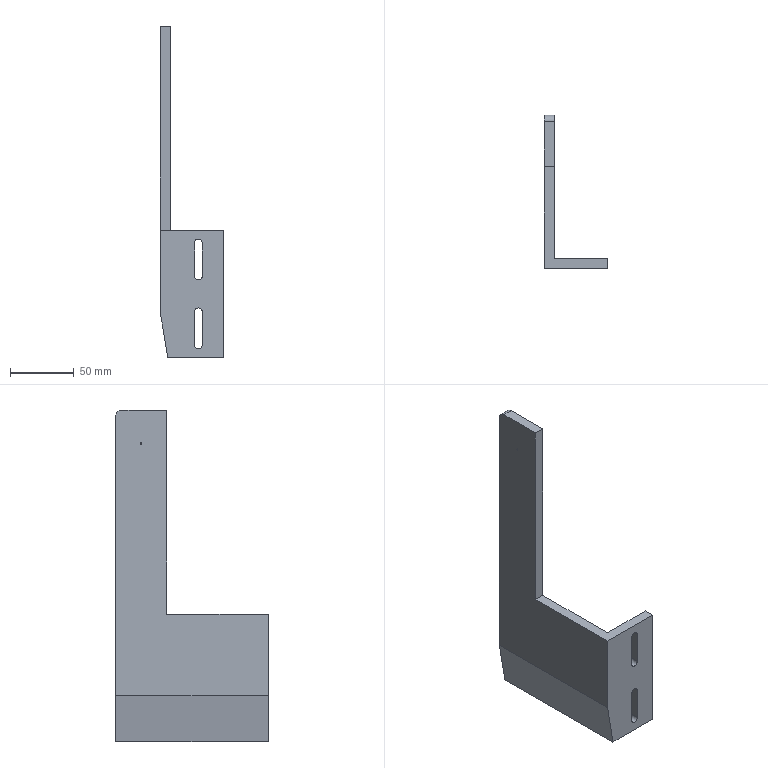Part | SolidWorks | features ICE 4, 3DProfileFeature 1, Extrusion 1, Fillet 1, HoleWzd 1 | 1 solid | 30 faces | box 50 x 120 x 260 mm | volume 164749 mm3 | plane 15 | cylinder 11 | cone 4 | commonest cylinder face diameters 6 x6 1.2 x2 4.2 x2 10 x1
STEP:
#1=CARTESIAN_POINT('',(0.,100.,234.6));
#2=VERTEX_POINT('',#1);
#3=CARTESIAN_POINT('',(0.,100.,233.4));
#4=VERTEX_POINT('',#3);
#5=CARTESIAN_POINT('',(0.,100.,234.));
#6=DIRECTION('',(1.,0.,0.));
#7=DIRECTION('',(0.,0.,-1.));
#8=AXIS2_PLACEMENT_3D('',#5,#6,#7);
#9=CIRCLE('',#8,0.6);
#10=EDGE_CURVE('',#2,#4,#9,.T.);
#11=ORIENTED_EDGE('',*,*,#10,.F.);
#12=CARTESIAN_POINT('',(8.,100.,234.6));
#13=VERTEX_POINT('',#12);
#14=CARTESIAN_POINT('',(0.,100.,234.6));
#15=DIRECTION('',(1.,0.,0.));
#16=VECTOR('',#15,1000.);
#17=LINE('',#14,#16);
#18=EDGE_CURVE('',#2,#13,#17,.T.);
#19=ORIENTED_EDGE('',*,*,#18,.T.);
#20=CARTESIAN_POINT('',(8.,100.,233.4));
#21=VERTEX_POINT('',#20);
#22=CARTESIAN_POINT('',(8.,100.,234.));
#23=DIRECTION('',(1.,0.,0.));
#24=DIRECTION('',(0.,0.,-1.));
#25=AXIS2_PLACEMENT_3D('',#22,#23,#24);
#26=CIRCLE('',#25,0.6);
#27=EDGE_CURVE('',#13,#21,#26,.T.);
#28=ORIENTED_EDGE('',*,*,#27,.T.);
#29=CARTESIAN_POINT('',(0.,100.,233.4));
#30=DIRECTION('',(1.,0.,0.));
#31=VECTOR('',#30,1000.);
#32=LINE('',#29,#31);
#33=EDGE_CURVE('',#4,#21,#32,.T.);
#34=ORIENTED_EDGE('',*,*,#33,.F.);
#35=EDGE_LOOP('',(#11,#19,#28,#34));
#36=FACE_OUTER_BOUND('',#35,.T.);
#37=CARTESIAN_POINT('',(0.,100.,234.));
#38=DIRECTION('',(1.,0.,0.));
#39=DIRECTION('',(0.,0.,-1.));
#40=AXIS2_PLACEMENT_3D('',#37,#38,#39);
#41=CYLINDRICAL_SURFACE('',#40,0.6);
#42=ADVANCED_FACE('',(#36),#41,.F.);
#43=CARTESIAN_POINT('',(7.575,75.,87.1));
#44=VERTEX_POINT('',#43);
#45=CARTESIAN_POINT('',(7.575,75.,82.9));
#46=VERTEX_POINT('',#45);
#47=CARTESIAN_POINT('',(7.575,75.,85.));
#48=DIRECTION('',(1.,0.,0.));
#49=DIRECTION('',(0.,0.,-1.));
#50=AXIS2_PLACEMENT_3D('',#47,#48,#49);
#51=CIRCLE('',#50,2.1);
#52=EDGE_CURVE('',#44,#46,#51,.T.);
#53=ORIENTED_EDGE('',*,*,#52,.F.);
#54=CARTESIAN_POINT('',(8.,75.,87.525));
#55=VERTEX_POINT('',#54);
#56=CARTESIAN_POINT('',(8.,75.,87.525));
#57=DIRECTION('',(0.7071,0.,0.7071));
#58=VECTOR('',#57,1000.);
#59=LINE('',#56,#58);
#60=EDGE_CURVE('',#44,#55,#59,.T.);
#61=ORIENTED_EDGE('',*,*,#60,.T.);
#62=CARTESIAN_POINT('',(8.,75.,82.475));
#63=VERTEX_POINT('',#62);
#64=CARTESIAN_POINT('',(8.,75.,85.));
#65=DIRECTION('',(1.,0.,0.));
#66=DIRECTION('',(0.,0.,-1.));
#67=AXIS2_PLACEMENT_3D('',#64,#65,#66);
#68=CIRCLE('',#67,2.525);
#69=EDGE_CURVE('',#55,#63,#68,.T.);
#70=ORIENTED_EDGE('',*,*,#69,.T.);
#71=CARTESIAN_POINT('',(8.,75.,82.475));
#72=DIRECTION('',(0.7071,0.,-0.7071));
#73=VECTOR('',#72,1000.);
#74=LINE('',#71,#73);
#75=EDGE_CURVE('',#46,#63,#74,.T.);
#76=ORIENTED_EDGE('',*,*,#75,.F.);
#77=EDGE_LOOP('',(#53,#61,#70,#76));
#78=FACE_OUTER_BOUND('',#77,.T.);
#79=CARTESIAN_POINT('',(8.,75.,85.));
#80=DIRECTION('',(1.,0.,0.));
#81=DIRECTION('',(0.,0.,-1.));
#82=AXIS2_PLACEMENT_3D('',#79,#80,#81);
#83=CONICAL_SURFACE('',#82,2.525,0.7854);
#84=ADVANCED_FACE('',(#78),#83,.F.);
#85=CARTESIAN_POINT('',(2.,75.,87.1));
#86=VERTEX_POINT('',#85);
#87=CARTESIAN_POINT('',(2.,75.,82.9));
#88=VERTEX_POINT('',#87);
#89=CARTESIAN_POINT('',(2.,75.,85.));
#90=DIRECTION('',(1.,0.,0.));
#91=DIRECTION('',(0.,0.,-1.));
#92=AXIS2_PLACEMENT_3D('',#89,#90,#91);
#93=CIRCLE('',#92,2.1);
#94=EDGE_CURVE('',#86,#88,#93,.T.);
#95=ORIENTED_EDGE('',*,*,#94,.F.);
#96=CARTESIAN_POINT('',(8.,75.,87.1));
#97=DIRECTION('',(1.,0.,0.));
#98=VECTOR('',#97,1000.);
#99=LINE('',#96,#98);
#100=EDGE_CURVE('',#86,#44,#99,.T.);
#101=ORIENTED_EDGE('',*,*,#100,.T.);
#102=ORIENTED_EDGE('',*,*,#52,.T.);
#103=CARTESIAN_POINT('',(8.,75.,82.9));
#104=DIRECTION('',(1.,0.,0.));
#105=VECTOR('',#104,1000.);
#106=LINE('',#103,#105);
#107=EDGE_CURVE('',#88,#46,#106,.T.);
#108=ORIENTED_EDGE('',*,*,#107,.F.);
#109=EDGE_LOOP('',(#95,#101,#102,#108));
#110=FACE_OUTER_BOUND('',#109,.T.);
#111=CARTESIAN_POINT('',(8.,75.,85.));
#112=DIRECTION('',(1.,0.,0.));
#113=DIRECTION('',(0.,0.,-1.));
#114=AXIS2_PLACEMENT_3D('',#111,#112,#113);
#115=CYLINDRICAL_SURFACE('',#114,2.1);
#116=ADVANCED_FACE('',(#110),#115,.F.);
#117=CARTESIAN_POINT('',(0.7382,75.,85.));
#118=VERTEX_POINT('',#117);
#119=CARTESIAN_POINT('',(2.,75.,82.9));
#120=DIRECTION('',(0.515,0.,-0.8572));
#121=VECTOR('',#120,1000.);
#122=LINE('',#119,#121);
#123=EDGE_CURVE('',#118,#88,#122,.T.);
#124=ORIENTED_EDGE('',*,*,#123,.F.);
#125=CARTESIAN_POINT('',(2.,75.,87.1));
#126=DIRECTION('',(0.515,0.,0.8572));
#127=VECTOR('',#126,1000.);
#128=LINE('',#125,#127);
#129=EDGE_CURVE('',#118,#86,#128,.T.);
#130=ORIENTED_EDGE('',*,*,#129,.T.);
#131=ORIENTED_EDGE('',*,*,#94,.T.);
#132=EDGE_LOOP('',(#124,#130,#131));
#133=FACE_OUTER_BOUND('',#132,.T.);
#134=CARTESIAN_POINT('',(2.,75.,85.));
#135=DIRECTION('',(1.,0.,0.));
#136=DIRECTION('',(0.,0.,-1.));
#137=AXIS2_PLACEMENT_3D('',#134,#135,#136);
#138=CONICAL_SURFACE('',#137,2.1,1.03);
#139=ADVANCED_FACE('',(#133),#138,.F.);
#140=CARTESIAN_POINT('',(30.,0.,39.));
#141=VERTEX_POINT('',#140);
#142=CARTESIAN_POINT('',(33.,0.,36.));
#143=VERTEX_POINT('',#142);
#144=CARTESIAN_POINT('',(30.,0.,36.));
#145=DIRECTION('',(0.,1.,0.));
#146=DIRECTION('',(0.,0.,1.));
#147=AXIS2_PLACEMENT_3D('',#144,#145,#146);
#148=CIRCLE('',#147,3.);
#149=EDGE_CURVE('',#141,#143,#148,.T.);
#150=ORIENTED_EDGE('',*,*,#149,.F.);
#151=CARTESIAN_POINT('',(30.,8.,39.));
#152=VERTEX_POINT('',#151);
#153=CARTESIAN_POINT('',(30.,-212.,39.));
#154=DIRECTION('',(0.,1.,0.));
#155=VECTOR('',#154,1000.);
#156=LINE('',#153,#155);
#157=EDGE_CURVE('',#141,#152,#156,.T.);
#158=ORIENTED_EDGE('',*,*,#157,.T.);
#159=CARTESIAN_POINT('',(33.,8.,36.));
#160=VERTEX_POINT('',#159);
#161=CARTESIAN_POINT('',(30.,8.,36.));
#162=DIRECTION('',(0.,1.,0.));
#163=DIRECTION('',(0.,0.,1.));
#164=AXIS2_PLACEMENT_3D('',#161,#162,#163);
#165=CIRCLE('',#164,3.);
#166=EDGE_CURVE('',#152,#160,#165,.T.);
#167=ORIENTED_EDGE('',*,*,#166,.T.);
#168=CARTESIAN_POINT('',(33.,-212.,36.));
#169=DIRECTION('',(0.,1.,0.));
#170=VECTOR('',#169,1000.);
#171=LINE('',#168,#170);
#172=EDGE_CURVE('',#143,#160,#171,.T.);
#173=ORIENTED_EDGE('',*,*,#172,.F.);
#174=EDGE_LOOP('',(#150,#158,#167,#173));
#175=FACE_OUTER_BOUND('',#174,.T.);
#176=CARTESIAN_POINT('',(30.,-212.,36.));
#177=DIRECTION('',(0.,1.,0.));
#178=DIRECTION('',(0.,0.,1.));
#179=AXIS2_PLACEMENT_3D('',#176,#177,#178);
#180=CYLINDRICAL_SURFACE('',#179,3.);
#181=ADVANCED_FACE('',(#175),#180,.F.);
#182=CARTESIAN_POINT('',(30.,0.,93.));
#183=VERTEX_POINT('',#182);
#184=CARTESIAN_POINT('',(33.,0.,90.));
#185=VERTEX_POINT('',#184);
#186=CARTESIAN_POINT('',(30.,0.,90.));
#187=DIRECTION('',(0.,1.,0.));
#188=DIRECTION('',(0.,0.,1.));
#189=AXIS2_PLACEMENT_3D('',#186,#187,#188);
#190=CIRCLE('',#189,3.);
#191=EDGE_CURVE('',#183,#185,#190,.T.);
#192=ORIENTED_EDGE('',*,*,#191,.F.);
#193=CARTESIAN_POINT('',(30.,8.,93.));
#194=VERTEX_POINT('',#193);
#195=CARTESIAN_POINT('',(30.,-212.,93.));
#196=DIRECTION('',(0.,1.,0.));
#197=VECTOR('',#196,1000.);
#198=LINE('',#195,#197);
#199=EDGE_CURVE('',#183,#194,#198,.T.);
#200=ORIENTED_EDGE('',*,*,#199,.T.);
#201=CARTESIAN_POINT('',(33.,8.,90.));
#202=VERTEX_POINT('',#201);
#203=CARTESIAN_POINT('',(30.,8.,90.));
#204=DIRECTION('',(0.,1.,0.));
#205=DIRECTION('',(0.,0.,1.));
#206=AXIS2_PLACEMENT_3D('',#203,#204,#205);
#207=CIRCLE('',#206,3.);
#208=EDGE_CURVE('',#194,#202,#207,.T.);
#209=ORIENTED_EDGE('',*,*,#208,.T.);
#210=CARTESIAN_POINT('',(33.,-212.,90.));
#211=DIRECTION('',(0.,1.,0.));
#212=VECTOR('',#211,1000.);
#213=LINE('',#210,#212);
#214=EDGE_CURVE('',#185,#202,#213,.T.);
#215=ORIENTED_EDGE('',*,*,#214,.F.);
#216=EDGE_LOOP('',(#192,#200,#209,#215));
#217=FACE_OUTER_BOUND('',#216,.T.);
#218=CARTESIAN_POINT('',(30.,-212.,90.));
#219=DIRECTION('',(0.,1.,0.));
#220=DIRECTION('',(0.,0.,1.));
#221=AXIS2_PLACEMENT_3D('',#218,#219,#220);
#222=CYLINDRICAL_SURFACE('',#221,3.);
#223=ADVANCED_FACE('',(#217),#222,.F.);
#224=CARTESIAN_POINT('',(27.,0.,10.));
#225=VERTEX_POINT('',#224);
#226=CARTESIAN_POINT('',(27.,0.,36.));
#227=VERTEX_POINT('',#226);
#228=CARTESIAN_POINT('',(27.,0.,260.));
#229=DIRECTION('',(0.,0.,1.));
#230=VECTOR('',#229,1000.);
#231=LINE('',#228,#230);
#232=EDGE_CURVE('',#225,#227,#231,.T.);
#233=ORIENTED_EDGE('',*,*,#232,.T.);
#234=CARTESIAN_POINT('',(30.,0.,36.));
#235=DIRECTION('',(0.,1.,0.));
#236=DIRECTION('',(0.,0.,1.));
#237=AXIS2_PLACEMENT_3D('',#234,#235,#236);
#238=CIRCLE('',#237,3.);
#239=EDGE_CURVE('',#227,#141,#238,.T.);
#240=ORIENTED_EDGE('',*,*,#239,.T.);
#241=ORIENTED_EDGE('',*,*,#149,.T.);
#242=CARTESIAN_POINT('',(33.,0.,10.));
#243=VERTEX_POINT('',#242);
#244=CARTESIAN_POINT('',(33.,0.,260.));
#245=DIRECTION('',(0.,0.,-1.));
#246=VECTOR('',#245,1000.);
#247=LINE('',#244,#246);
#248=EDGE_CURVE('',#143,#243,#247,.T.);
#249=ORIENTED_EDGE('',*,*,#248,.T.);
#250=CARTESIAN_POINT('',(30.,0.,10.));
#251=DIRECTION('',(0.,1.,0.));
#252=DIRECTION('',(0.,0.,1.));
#253=AXIS2_PLACEMENT_3D('',#250,#251,#252);
#254=CIRCLE('',#253,3.);
#255=EDGE_CURVE('',#243,#225,#254,.T.);
#256=ORIENTED_EDGE('',*,*,#255,.T.);
#257=EDGE_LOOP('',(#233,#240,#241,#249,#256));
#258=FACE_BOUND('',#257,.T.);
#259=CARTESIAN_POINT('',(27.,0.,64.));
#260=VERTEX_POINT('',#259);
#261=CARTESIAN_POINT('',(27.,0.,90.));
#262=VERTEX_POINT('',#261);
#263=CARTESIAN_POINT('',(27.,0.,260.));
#264=DIRECTION('',(0.,0.,1.));
#265=VECTOR('',#264,1000.);
#266=LINE('',#263,#265);
#267=EDGE_CURVE('',#260,#262,#266,.T.);
#268=ORIENTED_EDGE('',*,*,#267,.T.);
#269=CARTESIAN_POINT('',(30.,0.,90.));
#270=DIRECTION('',(0.,1.,0.));
#271=DIRECTION('',(0.,0.,1.));
#272=AXIS2_PLACEMENT_3D('',#269,#270,#271);
#273=CIRCLE('',#272,3.);
#274=EDGE_CURVE('',#262,#183,#273,.T.);
#275=ORIENTED_EDGE('',*,*,#274,.T.);
#276=ORIENTED_EDGE('',*,*,#191,.T.);
#277=CARTESIAN_POINT('',(33.,0.,64.));
#278=VERTEX_POINT('',#277);
#279=CARTESIAN_POINT('',(33.,0.,260.));
#280=DIRECTION('',(0.,0.,-1.));
#281=VECTOR('',#280,1000.);
#282=LINE('',#279,#281);
#283=EDGE_CURVE('',#185,#278,#282,.T.);
#284=ORIENTED_EDGE('',*,*,#283,.T.);
#285=CARTESIAN_POINT('',(30.,0.,64.));
#286=DIRECTION('',(0.,1.,0.));
#287=DIRECTION('',(0.,0.,1.));
#288=AXIS2_PLACEMENT_3D('',#285,#286,#287);
#289=CIRCLE('',#288,3.);
#290=EDGE_CURVE('',#278,#260,#289,.T.);
#291=ORIENTED_EDGE('',*,*,#290,.T.);
#292=EDGE_LOOP('',(#268,#275,#276,#284,#291));
#293=FACE_BOUND('',#292,.T.);
#294=CARTESIAN_POINT('',(0.,0.,100.));
#295=VERTEX_POINT('',#294);
#296=CARTESIAN_POINT('',(0.,0.,36.));
#297=VERTEX_POINT('',#296);
#298=CARTESIAN_POINT('',(0.,0.,260.));
#299=DIRECTION('',(0.,0.,-1.));
#300=VECTOR('',#299,1000.);
#301=LINE('',#298,#300);
#302=EDGE_CURVE('',#295,#297,#301,.T.);
#303=ORIENTED_EDGE('',*,*,#302,.T.);
#304=CARTESIAN_POINT('',(6.,0.,0.));
#305=VERTEX_POINT('',#304);
#306=CARTESIAN_POINT('',(6.,0.,0.));
#307=DIRECTION('',(0.1644,0.,-0.9864));
#308=VECTOR('',#307,1000.);
#309=LINE('',#306,#308);
#310=EDGE_CURVE('',#297,#305,#309,.T.);
#311=ORIENTED_EDGE('',*,*,#310,.T.);
#312=CARTESIAN_POINT('',(50.,0.,0.));
#313=VERTEX_POINT('',#312);
#314=CARTESIAN_POINT('',(0.,0.,0.));
#315=DIRECTION('',(1.,0.,0.));
#316=VECTOR('',#315,1000.);
#317=LINE('',#314,#316);
#318=EDGE_CURVE('',#305,#313,#317,.T.);
#319=ORIENTED_EDGE('',*,*,#318,.T.);
#320=CARTESIAN_POINT('',(50.,0.,100.));
#321=VERTEX_POINT('',#320);
#322=CARTESIAN_POINT('',(50.,0.,260.));
#323=DIRECTION('',(0.,0.,-1.));
#324=VECTOR('',#323,1000.);
#325=LINE('',#322,#324);
#326=EDGE_CURVE('',#321,#313,#325,.T.);
#327=ORIENTED_EDGE('',*,*,#326,.F.);
#328=CARTESIAN_POINT('',(0.,0.,100.));
#329=DIRECTION('',(1.,0.,0.));
#330=VECTOR('',#329,1000.);
#331=LINE('',#328,#330);
#332=EDGE_CURVE('',#295,#321,#331,.T.);
#333=ORIENTED_EDGE('',*,*,#332,.F.);
#334=EDGE_LOOP('',(#303,#311,#319,#327,#333));
#335=FACE_OUTER_BOUND('',#334,.T.);
#336=CARTESIAN_POINT('',(0.,0.,260.));
#337=DIRECTION('',(0.,1.,0.));
#338=DIRECTION('',(0.,0.,1.));
#339=AXIS2_PLACEMENT_3D('',#336,#337,#338);
#340=PLANE('',#339);
#341=ADVANCED_FACE('',(#258,#293,#335),#340,.F.);
#342=CARTESIAN_POINT('',(50.,8.,100.));
#343=VERTEX_POINT('',#342);
#344=CARTESIAN_POINT('',(50.,8.,0.));
#345=VERTEX_POINT('',#344);
#346=CARTESIAN_POINT('',(50.,8.,260.));
#347=DIRECTION('',(0.,0.,-1.));
#348=VECTOR('',#347,1000.);
#349=LINE('',#346,#348);
#350=EDGE_CURVE('',#343,#345,#349,.T.);
#351=ORIENTED_EDGE('',*,*,#350,.F.);
#352=CARTESIAN_POINT('',(50.,0.,100.));
#353=DIRECTION('',(0.,1.,0.));
#354=VECTOR('',#353,1000.);
#355=LINE('',#352,#354);
#356=EDGE_CURVE('',#321,#343,#355,.T.);
#357=ORIENTED_EDGE('',*,*,#356,.F.);
#358=ORIENTED_EDGE('',*,*,#326,.T.);
#359=CARTESIAN_POINT('',(50.,8.,0.));
#360=DIRECTION('',(0.,1.,0.));
#361=VECTOR('',#360,1000.);
#362=LINE('',#359,#361);
#363=EDGE_CURVE('',#313,#345,#362,.T.);
#364=ORIENTED_EDGE('',*,*,#363,.T.);
#365=EDGE_LOOP('',(#351,#357,#358,#364));
#366=FACE_OUTER_BOUND('',#365,.T.);
#367=CARTESIAN_POINT('',(50.,8.,260.));
#368=DIRECTION('',(-1.,0.,0.));
#369=DIRECTION('',(0.,0.,1.));
#370=AXIS2_PLACEMENT_3D('',#367,#368,#369);
#371=PLANE('',#370);
#372=ADVANCED_FACE('',(#366),#371,.F.);
#373=CARTESIAN_POINT('',(33.,8.,10.));
#374=VERTEX_POINT('',#373);
#375=CARTESIAN_POINT('',(33.,8.,36.));
#376=DIRECTION('',(0.,0.,-1.));
#377=VECTOR('',#376,1000.);
#378=LINE('',#375,#377);
#379=EDGE_CURVE('',#160,#374,#378,.T.);
#380=ORIENTED_EDGE('',*,*,#379,.F.);
#381=ORIENTED_EDGE('',*,*,#166,.F.);
#382=CARTESIAN_POINT('',(27.,8.,36.));
#383=VERTEX_POINT('',#382);
#384=CARTESIAN_POINT('',(30.,8.,36.));
#385=DIRECTION('',(0.,1.,0.));
#386=DIRECTION('',(0.,0.,1.));
#387=AXIS2_PLACEMENT_3D('',#384,#385,#386);
#388=CIRCLE('',#387,3.);
#389=EDGE_CURVE('',#383,#152,#388,.T.);
#390=ORIENTED_EDGE('',*,*,#389,.F.);
#391=CARTESIAN_POINT('',(27.,8.,10.));
#392=VERTEX_POINT('',#391);
#393=CARTESIAN_POINT('',(27.,8.,36.));
#394=DIRECTION('',(0.,0.,1.));
#395=VECTOR('',#394,1000.);
#396=LINE('',#393,#395);
#397=EDGE_CURVE('',#392,#383,#396,.T.);
#398=ORIENTED_EDGE('',*,*,#397,.F.);
#399=CARTESIAN_POINT('',(30.,8.,10.));
#400=DIRECTION('',(0.,1.,0.));
#401=DIRECTION('',(0.,0.,1.));
#402=AXIS2_PLACEMENT_3D('',#399,#400,#401);
#403=CIRCLE('',#402,3.);
#404=EDGE_CURVE('',#374,#392,#403,.T.);
#405=ORIENTED_EDGE('',*,*,#404,.F.);
#406=EDGE_LOOP('',(#380,#381,#390,#398,#405));
#407=FACE_BOUND('',#406,.T.);
#408=CARTESIAN_POINT('',(33.,8.,64.));
#409=VERTEX_POINT('',#408);
#410=CARTESIAN_POINT('',(33.,8.,90.));
#411=DIRECTION('',(0.,0.,-1.));
#412=VECTOR('',#411,1000.);
#413=LINE('',#410,#412);
#414=EDGE_CURVE('',#202,#409,#413,.T.);
#415=ORIENTED_EDGE('',*,*,#414,.F.);
#416=ORIENTED_EDGE('',*,*,#208,.F.);
#417=CARTESIAN_POINT('',(27.,8.,90.));
#418=VERTEX_POINT('',#417);
#419=CARTESIAN_POINT('',(30.,8.,90.));
#420=DIRECTION('',(0.,1.,0.));
#421=DIRECTION('',(0.,0.,1.));
#422=AXIS2_PLACEMENT_3D('',#419,#420,#421);
#423=CIRCLE('',#422,3.);
#424=EDGE_CURVE('',#418,#194,#423,.T.);
#425=ORIENTED_EDGE('',*,*,#424,.F.);
#426=CARTESIAN_POINT('',(27.,8.,64.));
#427=VERTEX_POINT('',#426);
#428=CARTESIAN_POINT('',(27.,8.,90.));
#429=DIRECTION('',(0.,0.,1.));
#430=VECTOR('',#429,1000.);
#431=LINE('',#428,#430);
#432=EDGE_CURVE('',#427,#418,#431,.T.);
#433=ORIENTED_EDGE('',*,*,#432,.F.);
#434=CARTESIAN_POINT('',(30.,8.,64.));
#435=DIRECTION('',(0.,1.,0.));
#436=DIRECTION('',(0.,0.,1.));
#437=AXIS2_PLACEMENT_3D('',#434,#435,#436);
#438=CIRCLE('',#437,3.);
#439=EDGE_CURVE('',#409,#427,#438,.T.);
#440=ORIENTED_EDGE('',*,*,#439,.F.);
#441=EDGE_LOOP('',(#415,#416,#425,#433,#440));
#442=FACE_BOUND('',#441,.T.);
#443=CARTESIAN_POINT('',(8.,8.,100.));
#444=VERTEX_POINT('',#443);
#445=CARTESIAN_POINT('',(8.,8.,0.));
#446=VERTEX_POINT('',#445);
#447=CARTESIAN_POINT('',(8.,8.,260.));
#448=DIRECTION('',(0.,0.,-1.));
#449=VECTOR('',#448,1000.);
#450=LINE('',#447,#449);
#451=EDGE_CURVE('',#444,#446,#450,.T.);
#452=ORIENTED_EDGE('',*,*,#451,.F.);
#453=CARTESIAN_POINT('',(8.,8.,100.));
#454=DIRECTION('',(1.,0.,0.));
#455=VECTOR('',#454,1000.);
#456=LINE('',#453,#455);
#457=EDGE_CURVE('',#444,#343,#456,.T.);
#458=ORIENTED_EDGE('',*,*,#457,.T.);
#459=ORIENTED_EDGE('',*,*,#350,.T.);
#460=CARTESIAN_POINT('',(8.,8.,0.));
#461=DIRECTION('',(-1.,0.,0.));
#462=VECTOR('',#461,1000.);
#463=LINE('',#460,#462);
#464=EDGE_CURVE('',#345,#446,#463,.T.);
#465=ORIENTED_EDGE('',*,*,#464,.T.);
#466=EDGE_LOOP('',(#452,#458,#459,#465));
#467=FACE_OUTER_BOUND('',#466,.T.);
#468=CARTESIAN_POINT('',(8.,8.,260.));
#469=DIRECTION('',(0.,-1.,0.));
#470=DIRECTION('',(0.,0.,-1.));
#471=AXIS2_PLACEMENT_3D('',#468,#469,#470);
#472=PLANE('',#471);
#473=ADVANCED_FACE('',(#407,#442,#467),#472,.F.);
#474=CARTESIAN_POINT('',(8.,100.,234.));
#475=DIRECTION('',(1.,0.,0.));
#476=DIRECTION('',(0.,0.,-1.));
#477=AXIS2_PLACEMENT_3D('',#474,#475,#476);
#478=CIRCLE('',#477,0.6);
#479=EDGE_CURVE('',#21,#13,#478,.T.);
#480=ORIENTED_EDGE('',*,*,#479,.F.);
#481=ORIENTED_EDGE('',*,*,#27,.F.);
#482=EDGE_LOOP('',(#480,#481));
#483=FACE_BOUND('',#482,.T.);
#484=CARTESIAN_POINT('',(8.,75.,85.));
#485=DIRECTION('',(1.,0.,0.));
#486=DIRECTION('',(0.,0.,-1.));
#487=AXIS2_PLACEMENT_3D('',#484,#485,#486);
#488=CIRCLE('',#487,2.525);
#489=EDGE_CURVE('',#63,#55,#488,.T.);
#490=ORIENTED_EDGE('',*,*,#489,.F.);
#491=ORIENTED_EDGE('',*,*,#69,.F.);
#492=EDGE_LOOP('',(#490,#491));
#493=FACE_BOUND('',#492,.T.);
#494=CARTESIAN_POINT('',(8.,120.,255.));
#495=VERTEX_POINT('',#494);
#496=CARTESIAN_POINT('',(8.,120.,0.));
#497=VERTEX_POINT('',#496);
#498=CARTESIAN_POINT('',(8.,120.,260.));
#499=DIRECTION('',(0.,0.,-1.));
#500=VECTOR('',#499,1000.);
#501=LINE('',#498,#500);
#502=EDGE_CURVE('',#495,#497,#501,.T.);
#503=ORIENTED_EDGE('',*,*,#502,.F.);
#504=CARTESIAN_POINT('',(8.,115.,260.));
#505=VERTEX_POINT('',#504);
#506=CARTESIAN_POINT('',(8.,115.,255.));
#507=DIRECTION('',(1.,0.,0.));
#508=DIRECTION('',(0.,0.,1.));
#509=AXIS2_PLACEMENT_3D('',#506,#507,#508);
#510=CIRCLE('',#509,5.);
#511=EDGE_CURVE('',#495,#505,#510,.T.);
#512=ORIENTED_EDGE('',*,*,#511,.T.);
#513=CARTESIAN_POINT('',(8.,80.,260.));
#514=VERTEX_POINT('',#513);
#515=CARTESIAN_POINT('',(8.,8.,260.));
#516=DIRECTION('',(0.,1.,0.));
#517=VECTOR('',#516,1000.);
#518=LINE('',#515,#517);
#519=EDGE_CURVE('',#514,#505,#518,.T.);
#520=ORIENTED_EDGE('',*,*,#519,.F.);
#521=CARTESIAN_POINT('',(8.,80.,100.));
#522=VERTEX_POINT('',#521);
#523=CARTESIAN_POINT('',(8.,80.,260.));
#524=DIRECTION('',(0.,0.,-1.));
#525=VECTOR('',#524,1000.);
#526=LINE('',#523,#525);
#527=EDGE_CURVE('',#514,#522,#526,.T.);
#528=ORIENTED_EDGE('',*,*,#527,.T.);
#529=CARTESIAN_POINT('',(8.,8.,100.));
#530=DIRECTION('',(0.,-1.,0.));
#531=VECTOR('',#530,1000.);
#532=LINE('',#529,#531);
#533=EDGE_CURVE('',#522,#444,#532,.T.);
#534=ORIENTED_EDGE('',*,*,#533,.T.);
#535=ORIENTED_EDGE('',*,*,#451,.T.);
#536=CARTESIAN_POINT('',(8.,8.,0.));
#537=DIRECTION('',(0.,1.,0.));
#538=VECTOR('',#537,1000.);
#539=LINE('',#536,#538);
#540=EDGE_CURVE('',#446,#497,#539,.T.);
#541=ORIENTED_EDGE('',*,*,#540,.T.);
#542=EDGE_LOOP('',(#503,#512,#520,#528,#534,#535,#541));
#543=FACE_OUTER_BOUND('',#542,.T.);
#544=CARTESIAN_POINT('',(8.,8.,260.));
#545=DIRECTION('',(-1.,0.,0.));
#546=DIRECTION('',(0.,0.,1.));
#547=AXIS2_PLACEMENT_3D('',#544,#545,#546);
#548=PLANE('',#547);
#549=ADVANCED_FACE('',(#483,#493,#543),#548,.F.);
#550=CARTESIAN_POINT('',(0.,120.,255.));
#551=VERTEX_POINT('',#550);
#552=CARTESIAN_POINT('',(0.,120.,36.));
#553=VERTEX_POINT('',#552);
#554=CARTESIAN_POINT('',(0.,120.,260.));
#555=DIRECTION('',(0.,0.,-1.));
#556=VECTOR('',#555,1000.);
#557=LINE('',#554,#556);
#558=EDGE_CURVE('',#551,#553,#557,.T.);
#559=ORIENTED_EDGE('',*,*,#558,.F.);
#560=CARTESIAN_POINT('',(8.,120.,255.));
#561=DIRECTION('',(1.,0.,0.));
#562=VECTOR('',#561,1000.);
#563=LINE('',#560,#562);
#564=EDGE_CURVE('',#551,#495,#563,.T.);
#565=ORIENTED_EDGE('',*,*,#564,.T.);
#566=ORIENTED_EDGE('',*,*,#502,.T.);
#567=CARTESIAN_POINT('',(6.,120.,0.));
#568=VERTEX_POINT('',#567);
#569=CARTESIAN_POINT('',(8.,120.,0.));
#570=DIRECTION('',(-1.,0.,0.));
#571=VECTOR('',#570,1000.);
#572=LINE('',#569,#571);
#573=EDGE_CURVE('',#497,#568,#572,.T.);
#574=ORIENTED_EDGE('',*,*,#573,.T.);
#575=CARTESIAN_POINT('',(6.,120.,0.));
#576=DIRECTION('',(0.1644,0.,-0.9864));
#577=VECTOR('',#576,1000.);
#578=LINE('',#575,#577);
#579=EDGE_CURVE('',#553,#568,#578,.T.);
#580=ORIENTED_EDGE('',*,*,#579,.F.);
#581=EDGE_LOOP('',(#559,#565,#566,#574,#580));
#582=FACE_OUTER_BOUND('',#581,.T.);
#583=CARTESIAN_POINT('',(8.,120.,260.));
#584=DIRECTION('',(0.,-1.,0.));
#585=DIRECTION('',(0.,0.,-1.));
#586=AXIS2_PLACEMENT_3D('',#583,#584,#585);
#587=PLANE('',#586);
#588=ADVANCED_FACE('',(#582),#587,.F.);
#589=CARTESIAN_POINT('',(0.,100.,234.));
#590=DIRECTION('',(1.,0.,0.));
#591=DIRECTION('',(0.,0.,-1.));
#592=AXIS2_PLACEMENT_3D('',#589,#590,#591);
#593=CIRCLE('',#592,0.6);
#594=EDGE_CURVE('',#4,#2,#593,.T.);
#595=ORIENTED_EDGE('',*,*,#594,.T.);
#596=ORIENTED_EDGE('',*,*,#10,.T.);
#597=EDGE_LOOP('',(#595,#596));
#598=FACE_BOUND('',#597,.T.);
#599=CARTESIAN_POINT('',(0.,115.,260.));
#600=VERTEX_POINT('',#599);
#601=CARTESIAN_POINT('',(0.,80.,260.));
#602=VERTEX_POINT('',#601);
#603=CARTESIAN_POINT('',(0.,0.,260.));
#604=DIRECTION('',(0.,-1.,0.));
#605=VECTOR('',#604,1000.);
#606=LINE('',#603,#605);
#607=EDGE_CURVE('',#600,#602,#606,.T.);
#608=ORIENTED_EDGE('',*,*,#607,.F.);
#609=CARTESIAN_POINT('',(0.,115.,255.));
#610=DIRECTION('',(-1.,0.,0.));
#611=DIRECTION('',(0.,0.,-1.));
#612=AXIS2_PLACEMENT_3D('',#609,#610,#611);
#613=CIRCLE('',#612,5.);
#614=EDGE_CURVE('',#600,#551,#613,.T.);
#615=ORIENTED_EDGE('',*,*,#614,.T.);
#616=ORIENTED_EDGE('',*,*,#558,.T.);
#617=CARTESIAN_POINT('',(0.,0.,36.));
#618=DIRECTION('',(0.,1.,0.));
#619=VECTOR('',#618,1000.);
#620=LINE('',#617,#619);
#621=EDGE_CURVE('',#297,#553,#620,.T.);
#622=ORIENTED_EDGE('',*,*,#621,.F.);
#623=ORIENTED_EDGE('',*,*,#302,.F.);
#624=CARTESIAN_POINT('',(0.,80.,100.));
#625=VERTEX_POINT('',#624);
#626=CARTESIAN_POINT('',(0.,0.,100.));
#627=DIRECTION('',(0.,1.,0.));
#628=VECTOR('',#627,1000.);
#629=LINE('',#626,#628);
#630=EDGE_CURVE('',#295,#625,#629,.T.);
#631=ORIENTED_EDGE('',*,*,#630,.T.);
#632=CARTESIAN_POINT('',(0.,80.,100.));
#633=DIRECTION('',(0.,0.,1.));
#634=VECTOR('',#633,1000.);
#635=LINE('',#632,#634);
#636=EDGE_CURVE('',#625,#602,#635,.T.);
#637=ORIENTED_EDGE('',*,*,#636,.T.);
#638=EDGE_LOOP('',(#608,#615,#616,#622,#623,#631,#637));
#639=FACE_OUTER_BOUND('',#638,.T.);
#640=CARTESIAN_POINT('',(0.,0.,260.));
#641=DIRECTION('',(1.,0.,0.));
#642=DIRECTION('',(0.,0.,-1.));
#643=AXIS2_PLACEMENT_3D('',#640,#641,#642);
#644=PLANE('',#643);
#645=ADVANCED_FACE('',(#598,#639),#644,.F.);
#646=ORIENTED_EDGE('',*,*,#519,.T.);
#647=CARTESIAN_POINT('',(0.,115.,260.));
#648=DIRECTION('',(-1.,0.,0.));
#649=VECTOR('',#648,1000.);
#650=LINE('',#647,#649);
#651=EDGE_CURVE('',#505,#600,#650,.T.);
#652=ORIENTED_EDGE('',*,*,#651,.T.);
#653=ORIENTED_EDGE('',*,*,#607,.T.);
#654=CARTESIAN_POINT('',(0.,80.,260.));
#655=DIRECTION('',(1.,0.,0.));
#656=VECTOR('',#655,1000.);
#657=LINE('',#654,#656);
#658=EDGE_CURVE('',#602,#514,#657,.T.);
#659=ORIENTED_EDGE('',*,*,#658,.T.);
#660=EDGE_LOOP('',(#646,#652,#653,#659));
#661=FACE_OUTER_BOUND('',#660,.T.);
#662=CARTESIAN_POINT('',(0.,0.,260.));
#663=DIRECTION('',(0.,0.,-1.));
#664=DIRECTION('',(-1.,0.,0.));
#665=AXIS2_PLACEMENT_3D('',#662,#663,#664);
#666=PLANE('',#665);
#667=ADVANCED_FACE('',(#661),#666,.F.);
#668=CARTESIAN_POINT('',(6.,0.,0.));
#669=DIRECTION('',(0.,1.,0.));
#670=VECTOR('',#669,1000.);
#671=LINE('',#668,#670);
#672=EDGE_CURVE('',#305,#568,#671,.T.);
#673=ORIENTED_EDGE('',*,*,#672,.T.);
#674=ORIENTED_EDGE('',*,*,#573,.F.);
#675=ORIENTED_EDGE('',*,*,#540,.F.);
#676=ORIENTED_EDGE('',*,*,#464,.F.);
#677=ORIENTED_EDGE('',*,*,#363,.F.);
#678=ORIENTED_EDGE('',*,*,#318,.F.);
#679=EDGE_LOOP('',(#673,#674,#675,#676,#677,#678));
#680=FACE_OUTER_BOUND('',#679,.T.);
#681=CARTESIAN_POINT('',(0.,0.,0.));
#682=DIRECTION('',(0.,0.,-1.));
#683=DIRECTION('',(-1.,0.,0.));
#684=AXIS2_PLACEMENT_3D('',#681,#682,#683);
#685=PLANE('',#684);
#686=ADVANCED_FACE('',(#680),#685,.T.);
#687=ORIENTED_EDGE('',*,*,#533,.F.);
#688=CARTESIAN_POINT('',(0.,80.,100.));
#689=DIRECTION('',(1.,0.,0.));
#690=VECTOR('',#689,1000.);
#691=LINE('',#688,#690);
#692=EDGE_CURVE('',#625,#522,#691,.T.);
#693=ORIENTED_EDGE('',*,*,#692,.F.);
#694=ORIENTED_EDGE('',*,*,#630,.F.);
#695=ORIENTED_EDGE('',*,*,#332,.T.);
#696=ORIENTED_EDGE('',*,*,#356,.T.);
#697=ORIENTED_EDGE('',*,*,#457,.F.);
#698=EDGE_LOOP('',(#687,#693,#694,#695,#696,#697));
#699=FACE_OUTER_BOUND('',#698,.T.);
#700=CARTESIAN_POINT('',(0.,0.,100.));
#701=DIRECTION('',(0.,0.,-1.));
#702=DIRECTION('',(-1.,0.,0.));
#703=AXIS2_PLACEMENT_3D('',#700,#701,#702);
#704=PLANE('',#703);
#705=ADVANCED_FACE('',(#699),#704,.F.);
#706=ORIENTED_EDGE('',*,*,#658,.F.);
#707=ORIENTED_EDGE('',*,*,#636,.F.);
#708=ORIENTED_EDGE('',*,*,#692,.T.);
#709=ORIENTED_EDGE('',*,*,#527,.F.);
#710=EDGE_LOOP('',(#706,#707,#708,#709));
#711=FACE_OUTER_BOUND('',#710,.T.);
#712=CARTESIAN_POINT('',(0.,80.,100.));
#713=DIRECTION('',(0.,1.,0.));
#714=DIRECTION('',(0.,0.,1.));
#715=AXIS2_PLACEMENT_3D('',#712,#713,#714);
#716=PLANE('',#715);
#717=ADVANCED_FACE('',(#711),#716,.F.);
#718=ORIENTED_EDGE('',*,*,#199,.F.);
#719=ORIENTED_EDGE('',*,*,#274,.F.);
#720=CARTESIAN_POINT('',(27.,-212.,90.));
#721=DIRECTION('',(0.,1.,0.));
#722=VECTOR('',#721,1000.);
#723=LINE('',#720,#722);
#724=EDGE_CURVE('',#262,#418,#723,.T.);
#725=ORIENTED_EDGE('',*,*,#724,.T.);
#726=ORIENTED_EDGE('',*,*,#424,.T.);
#727=EDGE_LOOP('',(#718,#719,#725,#726));
#728=FACE_OUTER_BOUND('',#727,.T.);
#729=CARTESIAN_POINT('',(30.,-212.,90.));
#730=DIRECTION('',(0.,1.,0.));
#731=DIRECTION('',(0.,0.,1.));
#732=AXIS2_PLACEMENT_3D('',#729,#730,#731);
#733=CYLINDRICAL_SURFACE('',#732,3.);
#734=ADVANCED_FACE('',(#728),#733,.F.);
#735=CARTESIAN_POINT('',(27.,-212.,64.));
#736=DIRECTION('',(0.,1.,0.));
#737=VECTOR('',#736,1000.);
#738=LINE('',#735,#737);
#739=EDGE_CURVE('',#260,#427,#738,.T.);
#740=ORIENTED_EDGE('',*,*,#739,.T.);
#741=ORIENTED_EDGE('',*,*,#432,.T.);
#742=ORIENTED_EDGE('',*,*,#724,.F.);
#743=ORIENTED_EDGE('',*,*,#267,.F.);
#744=EDGE_LOOP('',(#740,#741,#742,#743));
#745=FACE_OUTER_BOUND('',#744,.T.);
#746=CARTESIAN_POINT('',(27.,-212.,90.));
#747=DIRECTION('',(-1.,0.,0.));
#748=DIRECTION('',(0.,0.,1.));
#749=AXIS2_PLACEMENT_3D('',#746,#747,#748);
#750=PLANE('',#749);
#751=ADVANCED_FACE('',(#745),#750,.F.);
#752=CARTESIAN_POINT('',(33.,-212.,64.));
#753=DIRECTION('',(0.,1.,0.));
#754=VECTOR('',#753,1000.);
#755=LINE('',#752,#754);
#756=EDGE_CURVE('',#278,#409,#755,.T.);
#757=ORIENTED_EDGE('',*,*,#756,.T.);
#758=ORIENTED_EDGE('',*,*,#439,.T.);
#759=ORIENTED_EDGE('',*,*,#739,.F.);
#760=ORIENTED_EDGE('',*,*,#290,.F.);
#761=EDGE_LOOP('',(#757,#758,#759,#760));
#762=FACE_OUTER_BOUND('',#761,.T.);
#763=CARTESIAN_POINT('',(30.,-212.,64.));
#764=DIRECTION('',(0.,1.,0.));
#765=DIRECTION('',(0.,0.,1.));
#766=AXIS2_PLACEMENT_3D('',#763,#764,#765);
#767=CYLINDRICAL_SURFACE('',#766,3.);
#768=ADVANCED_FACE('',(#762),#767,.F.);
#769=ORIENTED_EDGE('',*,*,#214,.T.);
#770=ORIENTED_EDGE('',*,*,#414,.T.);
#771=ORIENTED_EDGE('',*,*,#756,.F.);
#772=ORIENTED_EDGE('',*,*,#283,.F.);
#773=EDGE_LOOP('',(#769,#770,#771,#772));
#774=FACE_OUTER_BOUND('',#773,.T.);
#775=CARTESIAN_POINT('',(33.,-212.,90.));
#776=DIRECTION('',(1.,0.,0.));
#777=DIRECTION('',(0.,0.,-1.));
#778=AXIS2_PLACEMENT_3D('',#775,#776,#777);
#779=PLANE('',#778);
#780=ADVANCED_FACE('',(#774),#779,.F.);
#781=ORIENTED_EDGE('',*,*,#157,.F.);
#782=ORIENTED_EDGE('',*,*,#239,.F.);
#783=CARTESIAN_POINT('',(27.,-212.,36.));
#784=DIRECTION('',(0.,1.,0.));
#785=VECTOR('',#784,1000.);
#786=LINE('',#783,#785);
#787=EDGE_CURVE('',#227,#383,#786,.T.);
#788=ORIENTED_EDGE('',*,*,#787,.T.);
#789=ORIENTED_EDGE('',*,*,#389,.T.);
#790=EDGE_LOOP('',(#781,#782,#788,#789));
#791=FACE_OUTER_BOUND('',#790,.T.);
#792=CARTESIAN_POINT('',(30.,-212.,36.));
#793=DIRECTION('',(0.,1.,0.));
#794=DIRECTION('',(0.,0.,1.));
#795=AXIS2_PLACEMENT_3D('',#792,#793,#794);
#796=CYLINDRICAL_SURFACE('',#795,3.);
#797=ADVANCED_FACE('',(#791),#796,.F.);
#798=CARTESIAN_POINT('',(27.,-212.,10.));
#799=DIRECTION('',(0.,1.,0.));
#800=VECTOR('',#799,1000.);
#801=LINE('',#798,#800);
#802=EDGE_CURVE('',#225,#392,#801,.T.);
#803=ORIENTED_EDGE('',*,*,#802,.T.);
#804=ORIENTED_EDGE('',*,*,#397,.T.);
#805=ORIENTED_EDGE('',*,*,#787,.F.);
#806=ORIENTED_EDGE('',*,*,#232,.F.);
#807=EDGE_LOOP('',(#803,#804,#805,#806));
#808=FACE_OUTER_BOUND('',#807,.T.);
#809=CARTESIAN_POINT('',(27.,-212.,36.));
#810=DIRECTION('',(-1.,0.,0.));
#811=DIRECTION('',(0.,0.,1.));
#812=AXIS2_PLACEMENT_3D('',#809,#810,#811);
#813=PLANE('',#812);
#814=ADVANCED_FACE('',(#808),#813,.F.);
#815=CARTESIAN_POINT('',(33.,-212.,10.));
#816=DIRECTION('',(0.,1.,0.));
#817=VECTOR('',#816,1000.);
#818=LINE('',#815,#817);
#819=EDGE_CURVE('',#243,#374,#818,.T.);
#820=ORIENTED_EDGE('',*,*,#819,.T.);
#821=ORIENTED_EDGE('',*,*,#404,.T.);
#822=ORIENTED_EDGE('',*,*,#802,.F.);
#823=ORIENTED_EDGE('',*,*,#255,.F.);
#824=EDGE_LOOP('',(#820,#821,#822,#823));
#825=FACE_OUTER_BOUND('',#824,.T.);
#826=CARTESIAN_POINT('',(30.,-212.,10.));
#827=DIRECTION('',(0.,1.,0.));
#828=DIRECTION('',(0.,0.,1.));
#829=AXIS2_PLACEMENT_3D('',#826,#827,#828);
#830=CYLINDRICAL_SURFACE('',#829,3.);
#831=ADVANCED_FACE('',(#825),#830,.F.);
#832=ORIENTED_EDGE('',*,*,#172,.T.);
#833=ORIENTED_EDGE('',*,*,#379,.T.);
#834=ORIENTED_EDGE('',*,*,#819,.F.);
#835=ORIENTED_EDGE('',*,*,#248,.F.);
#836=EDGE_LOOP('',(#832,#833,#834,#835));
#837=FACE_OUTER_BOUND('',#836,.T.);
#838=CARTESIAN_POINT('',(33.,-212.,36.));
#839=DIRECTION('',(1.,0.,0.));
#840=DIRECTION('',(0.,0.,-1.));
#841=AXIS2_PLACEMENT_3D('',#838,#839,#840);
#842=PLANE('',#841);
#843=ADVANCED_FACE('',(#837),#842,.F.);
#844=ORIENTED_EDGE('',*,*,#579,.T.);
#845=ORIENTED_EDGE('',*,*,#672,.F.);
#846=ORIENTED_EDGE('',*,*,#310,.F.);
#847=ORIENTED_EDGE('',*,*,#621,.T.);
#848=EDGE_LOOP('',(#844,#845,#846,#847));
#849=FACE_OUTER_BOUND('',#848,.T.);
#850=CARTESIAN_POINT('',(6.,0.,0.));
#851=DIRECTION('',(0.9864,0.,0.1644));
#852=DIRECTION('',(0.1644,0.,-0.9864));
#853=AXIS2_PLACEMENT_3D('',#850,#851,#852);
#854=PLANE('',#853);
#855=ADVANCED_FACE('',(#849),#854,.F.);
#856=ORIENTED_EDGE('',*,*,#129,.F.);
#857=ORIENTED_EDGE('',*,*,#123,.T.);
#858=CARTESIAN_POINT('',(2.,75.,85.));
#859=DIRECTION('',(1.,0.,0.));
#860=DIRECTION('',(0.,0.,-1.));
#861=AXIS2_PLACEMENT_3D('',#858,#859,#860);
#862=CIRCLE('',#861,2.1);
#863=EDGE_CURVE('',#88,#86,#862,.T.);
#864=ORIENTED_EDGE('',*,*,#863,.T.);
#865=EDGE_LOOP('',(#856,#857,#864));
#866=FACE_OUTER_BOUND('',#865,.T.);
#867=CARTESIAN_POINT('',(2.,75.,85.));
#868=DIRECTION('',(1.,0.,0.));
#869=DIRECTION('',(0.,0.,-1.));
#870=AXIS2_PLACEMENT_3D('',#867,#868,#869);
#871=CONICAL_SURFACE('',#870,2.1,1.03);
#872=ADVANCED_FACE('',(#866),#871,.F.);
#873=ORIENTED_EDGE('',*,*,#100,.F.);
#874=ORIENTED_EDGE('',*,*,#863,.F.);
#875=ORIENTED_EDGE('',*,*,#107,.T.);
#876=CARTESIAN_POINT('',(7.575,75.,85.));
#877=DIRECTION('',(1.,0.,0.));
#878=DIRECTION('',(0.,0.,-1.));
#879=AXIS2_PLACEMENT_3D('',#876,#877,#878);
#880=CIRCLE('',#879,2.1);
#881=EDGE_CURVE('',#46,#44,#880,.T.);
#882=ORIENTED_EDGE('',*,*,#881,.T.);
#883=EDGE_LOOP('',(#873,#874,#875,#882));
#884=FACE_OUTER_BOUND('',#883,.T.);
#885=CARTESIAN_POINT('',(8.,75.,85.));
#886=DIRECTION('',(1.,0.,0.));
#887=DIRECTION('',(0.,0.,-1.));
#888=AXIS2_PLACEMENT_3D('',#885,#886,#887);
#889=CYLINDRICAL_SURFACE('',#888,2.1);
#890=ADVANCED_FACE('',(#884),#889,.F.);
#891=ORIENTED_EDGE('',*,*,#60,.F.);
#892=ORIENTED_EDGE('',*,*,#881,.F.);
#893=ORIENTED_EDGE('',*,*,#75,.T.);
#894=ORIENTED_EDGE('',*,*,#489,.T.);
#895=EDGE_LOOP('',(#891,#892,#893,#894));
#896=FACE_OUTER_BOUND('',#895,.T.);
#897=CARTESIAN_POINT('',(8.,75.,85.));
#898=DIRECTION('',(1.,0.,0.));
#899=DIRECTION('',(0.,0.,-1.));
#900=AXIS2_PLACEMENT_3D('',#897,#898,#899);
#901=CONICAL_SURFACE('',#900,2.525,0.7854);
#902=ADVANCED_FACE('',(#896),#901,.F.);
#903=ORIENTED_EDGE('',*,*,#511,.F.);
#904=ORIENTED_EDGE('',*,*,#564,.F.);
#905=ORIENTED_EDGE('',*,*,#614,.F.);
#906=ORIENTED_EDGE('',*,*,#651,.F.);
#907=EDGE_LOOP('',(#903,#904,#905,#906));
#908=FACE_OUTER_BOUND('',#907,.T.);
#909=CARTESIAN_POINT('',(0.,115.,255.));
#910=DIRECTION('',(-1.,0.,0.));
#911=DIRECTION('',(0.,0.,1.));
#912=AXIS2_PLACEMENT_3D('',#909,#910,#911);
#913=CYLINDRICAL_SURFACE('',#912,5.);
#914=ADVANCED_FACE('',(#908),#913,.T.);
#915=ORIENTED_EDGE('',*,*,#18,.F.);
#916=ORIENTED_EDGE('',*,*,#594,.F.);
#917=ORIENTED_EDGE('',*,*,#33,.T.);
#918=ORIENTED_EDGE('',*,*,#479,.T.);
#919=EDGE_LOOP('',(#915,#916,#917,#918));
#920=FACE_OUTER_BOUND('',#919,.T.);
#921=CARTESIAN_POINT('',(0.,100.,234.));
#922=DIRECTION('',(1.,0.,0.));
#923=DIRECTION('',(0.,0.,-1.));
#924=AXIS2_PLACEMENT_3D('',#921,#922,#923);
#925=CYLINDRICAL_SURFACE('',#924,0.6);
#926=ADVANCED_FACE('',(#920),#925,.F.);
#927=CLOSED_SHELL('',(#42,#84,#116,#139,#181,#223,#341,#372,#473,#549,#588,#645,#667,#686,#705,#717,#734,#751,#768,#780,#797,#814,#831,#843,#855,#872,#890,#902,#914,#926));
#928=MANIFOLD_SOLID_BREP('',#927);
#929=CARTESIAN_POINT('',(0.,0.,0.));
#930=DIRECTION('',(0.,0.,1.));
#931=DIRECTION('',(1.,0.,0.));
#932=AXIS2_PLACEMENT_3D('',#929,#930,#931);
#933=(LENGTH_UNIT()NAMED_UNIT(*)SI_UNIT(.MILLI.,.METRE.));
#934=UNCERTAINTY_MEASURE_WITH_UNIT(LENGTH_MEASURE(0.00001),#933,'','');
#935=(NAMED_UNIT(*)PLANE_ANGLE_UNIT()SI_UNIT($,.RADIAN.));
#936=(NAMED_UNIT(*)SI_UNIT($,.STERADIAN.)SOLID_ANGLE_UNIT());
#937=(GEOMETRIC_REPRESENTATION_CONTEXT(3)GLOBAL_UNCERTAINTY_ASSIGNED_CONTEXT((#934))GLOBAL_UNIT_ASSIGNED_CONTEXT((#933,#935,#936))REPRESENTATION_CONTEXT('',''));
#938=ADVANCED_BREP_SHAPE_REPRESENTATION('',(#928,#932),#937);